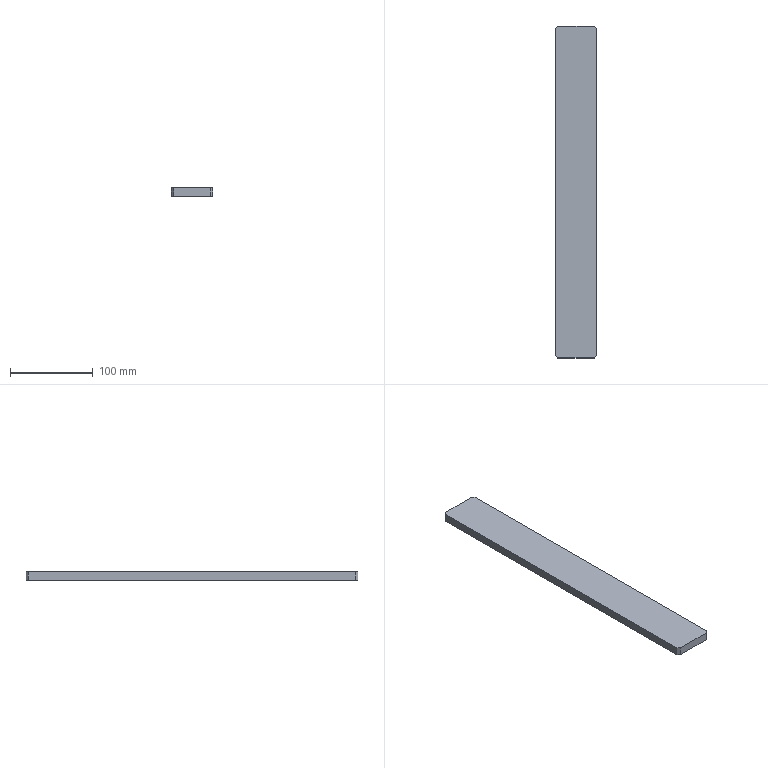Part | SolidWorks | features Chamfer 1, Extrusion 1 | 1 solid | 10 faces | box 50 x 400 x 10 mm | volume 199820 mm3 | plane 10
STEP:
#1=CARTESIAN_POINT('',(-128.557,546.194,0.));
#2=VERTEX_POINT('',#1);
#3=CARTESIAN_POINT('',(-128.557,152.194,0.));
#4=VERTEX_POINT('',#3);
#5=CARTESIAN_POINT('',(-128.557,549.194,0.));
#6=DIRECTION('',(0.,-1.,0.));
#7=VECTOR('',#6,1000.);
#8=LINE('',#5,#7);
#9=EDGE_CURVE('',#2,#4,#8,.T.);
#10=ORIENTED_EDGE('',*,*,#9,.T.);
#11=CARTESIAN_POINT('',(-128.557,152.194,10.));
#12=VERTEX_POINT('',#11);
#13=CARTESIAN_POINT('',(-128.557,152.194,10.));
#14=DIRECTION('',(0.,0.,1.));
#15=VECTOR('',#14,1000.);
#16=LINE('',#13,#15);
#17=EDGE_CURVE('',#4,#12,#16,.T.);
#18=ORIENTED_EDGE('',*,*,#17,.T.);
#19=CARTESIAN_POINT('',(-128.557,546.194,10.));
#20=VERTEX_POINT('',#19);
#21=CARTESIAN_POINT('',(-128.557,549.194,10.));
#22=DIRECTION('',(0.,-1.,0.));
#23=VECTOR('',#22,1000.);
#24=LINE('',#21,#23);
#25=EDGE_CURVE('',#20,#12,#24,.T.);
#26=ORIENTED_EDGE('',*,*,#25,.F.);
#27=CARTESIAN_POINT('',(-128.557,546.194,10.));
#28=DIRECTION('',(0.,0.,-1.));
#29=VECTOR('',#28,1000.);
#30=LINE('',#27,#29);
#31=EDGE_CURVE('',#20,#2,#30,.T.);
#32=ORIENTED_EDGE('',*,*,#31,.T.);
#33=EDGE_LOOP('',(#10,#18,#26,#32));
#34=FACE_OUTER_BOUND('',#33,.T.);
#35=CARTESIAN_POINT('',(-128.557,549.194,10.));
#36=DIRECTION('',(1.,0.,0.));
#37=DIRECTION('',(0.,1.,0.));
#38=AXIS2_PLACEMENT_3D('',#35,#36,#37);
#39=PLANE('',#38);
#40=ADVANCED_FACE('',(#34),#39,.F.);
#41=CARTESIAN_POINT('',(-125.557,149.194,0.));
#42=VERTEX_POINT('',#41);
#43=CARTESIAN_POINT('',(-81.557,149.194,0.));
#44=VERTEX_POINT('',#43);
#45=CARTESIAN_POINT('',(-128.557,149.194,0.));
#46=DIRECTION('',(1.,0.,0.));
#47=VECTOR('',#46,1000.);
#48=LINE('',#45,#47);
#49=EDGE_CURVE('',#42,#44,#48,.T.);
#50=ORIENTED_EDGE('',*,*,#49,.T.);
#51=CARTESIAN_POINT('',(-81.557,149.194,10.));
#52=VERTEX_POINT('',#51);
#53=CARTESIAN_POINT('',(-81.557,149.194,10.));
#54=DIRECTION('',(0.,0.,1.));
#55=VECTOR('',#54,1000.);
#56=LINE('',#53,#55);
#57=EDGE_CURVE('',#44,#52,#56,.T.);
#58=ORIENTED_EDGE('',*,*,#57,.T.);
#59=CARTESIAN_POINT('',(-125.557,149.194,10.));
#60=VERTEX_POINT('',#59);
#61=CARTESIAN_POINT('',(-128.557,149.194,10.));
#62=DIRECTION('',(1.,0.,0.));
#63=VECTOR('',#62,1000.);
#64=LINE('',#61,#63);
#65=EDGE_CURVE('',#60,#52,#64,.T.);
#66=ORIENTED_EDGE('',*,*,#65,.F.);
#67=CARTESIAN_POINT('',(-125.557,149.194,10.));
#68=DIRECTION('',(0.,0.,-1.));
#69=VECTOR('',#68,1000.);
#70=LINE('',#67,#69);
#71=EDGE_CURVE('',#60,#42,#70,.T.);
#72=ORIENTED_EDGE('',*,*,#71,.T.);
#73=EDGE_LOOP('',(#50,#58,#66,#72));
#74=FACE_OUTER_BOUND('',#73,.T.);
#75=CARTESIAN_POINT('',(-128.557,149.194,10.));
#76=DIRECTION('',(0.,1.,0.));
#77=DIRECTION('',(0.,0.,1.));
#78=AXIS2_PLACEMENT_3D('',#75,#76,#77);
#79=PLANE('',#78);
#80=ADVANCED_FACE('',(#74),#79,.F.);
#81=CARTESIAN_POINT('',(-78.557,152.194,10.));
#82=VERTEX_POINT('',#81);
#83=CARTESIAN_POINT('',(-78.557,546.194,10.));
#84=VERTEX_POINT('',#83);
#85=CARTESIAN_POINT('',(-78.557,549.194,10.));
#86=DIRECTION('',(0.,1.,0.));
#87=VECTOR('',#86,1000.);
#88=LINE('',#85,#87);
#89=EDGE_CURVE('',#82,#84,#88,.T.);
#90=ORIENTED_EDGE('',*,*,#89,.F.);
#91=CARTESIAN_POINT('',(-78.557,152.194,0.));
#92=VERTEX_POINT('',#91);
#93=CARTESIAN_POINT('',(-78.557,152.194,10.));
#94=DIRECTION('',(0.,0.,-1.));
#95=VECTOR('',#94,1000.);
#96=LINE('',#93,#95);
#97=EDGE_CURVE('',#82,#92,#96,.T.);
#98=ORIENTED_EDGE('',*,*,#97,.T.);
#99=CARTESIAN_POINT('',(-78.557,546.194,0.));
#100=VERTEX_POINT('',#99);
#101=CARTESIAN_POINT('',(-78.557,549.194,0.));
#102=DIRECTION('',(0.,1.,0.));
#103=VECTOR('',#102,1000.);
#104=LINE('',#101,#103);
#105=EDGE_CURVE('',#92,#100,#104,.T.);
#106=ORIENTED_EDGE('',*,*,#105,.T.);
#107=CARTESIAN_POINT('',(-78.557,546.194,10.));
#108=DIRECTION('',(0.,0.,1.));
#109=VECTOR('',#108,1000.);
#110=LINE('',#107,#109);
#111=EDGE_CURVE('',#100,#84,#110,.T.);
#112=ORIENTED_EDGE('',*,*,#111,.T.);
#113=EDGE_LOOP('',(#90,#98,#106,#112));
#114=FACE_OUTER_BOUND('',#113,.T.);
#115=CARTESIAN_POINT('',(-78.557,549.194,10.));
#116=DIRECTION('',(-1.,0.,0.));
#117=DIRECTION('',(0.,-1.,0.));
#118=AXIS2_PLACEMENT_3D('',#115,#116,#117);
#119=PLANE('',#118);
#120=ADVANCED_FACE('',(#114),#119,.F.);
#121=CARTESIAN_POINT('',(-81.557,549.194,0.));
#122=VERTEX_POINT('',#121);
#123=CARTESIAN_POINT('',(-125.557,549.194,0.));
#124=VERTEX_POINT('',#123);
#125=CARTESIAN_POINT('',(-128.557,549.194,0.));
#126=DIRECTION('',(-1.,0.,0.));
#127=VECTOR('',#126,1000.);
#128=LINE('',#125,#127);
#129=EDGE_CURVE('',#122,#124,#128,.T.);
#130=ORIENTED_EDGE('',*,*,#129,.T.);
#131=CARTESIAN_POINT('',(-125.557,549.194,10.));
#132=VERTEX_POINT('',#131);
#133=CARTESIAN_POINT('',(-125.557,549.194,10.));
#134=DIRECTION('',(0.,0.,1.));
#135=VECTOR('',#134,1000.);
#136=LINE('',#133,#135);
#137=EDGE_CURVE('',#124,#132,#136,.T.);
#138=ORIENTED_EDGE('',*,*,#137,.T.);
#139=CARTESIAN_POINT('',(-81.557,549.194,10.));
#140=VERTEX_POINT('',#139);
#141=CARTESIAN_POINT('',(-128.557,549.194,10.));
#142=DIRECTION('',(-1.,0.,0.));
#143=VECTOR('',#142,1000.);
#144=LINE('',#141,#143);
#145=EDGE_CURVE('',#140,#132,#144,.T.);
#146=ORIENTED_EDGE('',*,*,#145,.F.);
#147=CARTESIAN_POINT('',(-81.557,549.194,10.));
#148=DIRECTION('',(0.,0.,-1.));
#149=VECTOR('',#148,1000.);
#150=LINE('',#147,#149);
#151=EDGE_CURVE('',#140,#122,#150,.T.);
#152=ORIENTED_EDGE('',*,*,#151,.T.);
#153=EDGE_LOOP('',(#130,#138,#146,#152));
#154=FACE_OUTER_BOUND('',#153,.T.);
#155=CARTESIAN_POINT('',(-128.557,549.194,10.));
#156=DIRECTION('',(0.,-1.,0.));
#157=DIRECTION('',(0.,0.,-1.));
#158=AXIS2_PLACEMENT_3D('',#155,#156,#157);
#159=PLANE('',#158);
#160=ADVANCED_FACE('',(#154),#159,.F.);
#161=ORIENTED_EDGE('',*,*,#65,.T.);
#162=CARTESIAN_POINT('',(-115.375,115.375,10.));
#163=DIRECTION('',(0.7071,0.7071,0.));
#164=VECTOR('',#163,1000.);
#165=LINE('',#162,#164);
#166=EDGE_CURVE('',#52,#82,#165,.T.);
#167=ORIENTED_EDGE('',*,*,#166,.T.);
#168=ORIENTED_EDGE('',*,*,#89,.T.);
#169=CARTESIAN_POINT('',(233.818,233.818,10.));
#170=DIRECTION('',(-0.7071,0.7071,0.));
#171=VECTOR('',#170,1000.);
#172=LINE('',#169,#171);
#173=EDGE_CURVE('',#84,#140,#172,.T.);
#174=ORIENTED_EDGE('',*,*,#173,.T.);
#175=ORIENTED_EDGE('',*,*,#145,.T.);
#176=CARTESIAN_POINT('',(-337.375,337.375,10.));
#177=DIRECTION('',(-0.7071,-0.7071,0.));
#178=VECTOR('',#177,1000.);
#179=LINE('',#176,#178);
#180=EDGE_CURVE('',#132,#20,#179,.T.);
#181=ORIENTED_EDGE('',*,*,#180,.T.);
#182=ORIENTED_EDGE('',*,*,#25,.T.);
#183=CARTESIAN_POINT('',(11.818,11.818,10.));
#184=DIRECTION('',(0.7071,-0.7071,0.));
#185=VECTOR('',#184,1000.);
#186=LINE('',#183,#185);
#187=EDGE_CURVE('',#12,#60,#186,.T.);
#188=ORIENTED_EDGE('',*,*,#187,.T.);
#189=EDGE_LOOP('',(#161,#167,#168,#174,#175,#181,#182,#188));
#190=FACE_OUTER_BOUND('',#189,.T.);
#191=CARTESIAN_POINT('',(0.,0.,10.));
#192=DIRECTION('',(0.,0.,1.));
#193=DIRECTION('',(1.,0.,0.));
#194=AXIS2_PLACEMENT_3D('',#191,#192,#193);
#195=PLANE('',#194);
#196=ADVANCED_FACE('',(#190),#195,.T.);
#197=ORIENTED_EDGE('',*,*,#105,.F.);
#198=CARTESIAN_POINT('',(-78.557,152.194,0.));
#199=DIRECTION('',(-0.7071,-0.7071,0.));
#200=VECTOR('',#199,1000.);
#201=LINE('',#198,#200);
#202=EDGE_CURVE('',#92,#44,#201,.T.);
#203=ORIENTED_EDGE('',*,*,#202,.T.);
#204=ORIENTED_EDGE('',*,*,#49,.F.);
#205=CARTESIAN_POINT('',(-125.557,149.194,0.));
#206=DIRECTION('',(-0.7071,0.7071,0.));
#207=VECTOR('',#206,1000.);
#208=LINE('',#205,#207);
#209=EDGE_CURVE('',#42,#4,#208,.T.);
#210=ORIENTED_EDGE('',*,*,#209,.T.);
#211=ORIENTED_EDGE('',*,*,#9,.F.);
#212=CARTESIAN_POINT('',(-128.557,546.194,0.));
#213=DIRECTION('',(0.7071,0.7071,0.));
#214=VECTOR('',#213,1000.);
#215=LINE('',#212,#214);
#216=EDGE_CURVE('',#2,#124,#215,.T.);
#217=ORIENTED_EDGE('',*,*,#216,.T.);
#218=ORIENTED_EDGE('',*,*,#129,.F.);
#219=CARTESIAN_POINT('',(-81.557,549.194,0.));
#220=DIRECTION('',(0.7071,-0.7071,0.));
#221=VECTOR('',#220,1000.);
#222=LINE('',#219,#221);
#223=EDGE_CURVE('',#122,#100,#222,.T.);
#224=ORIENTED_EDGE('',*,*,#223,.T.);
#225=EDGE_LOOP('',(#197,#203,#204,#210,#211,#217,#218,#224));
#226=FACE_OUTER_BOUND('',#225,.T.);
#227=CARTESIAN_POINT('',(0.,0.,0.));
#228=DIRECTION('',(0.,0.,1.));
#229=DIRECTION('',(1.,0.,0.));
#230=AXIS2_PLACEMENT_3D('',#227,#228,#229);
#231=PLANE('',#230);
#232=ADVANCED_FACE('',(#226),#231,.F.);
#233=ORIENTED_EDGE('',*,*,#166,.F.);
#234=ORIENTED_EDGE('',*,*,#57,.F.);
#235=ORIENTED_EDGE('',*,*,#202,.F.);
#236=ORIENTED_EDGE('',*,*,#97,.F.);
#237=EDGE_LOOP('',(#233,#234,#235,#236));
#238=FACE_OUTER_BOUND('',#237,.T.);
#239=CARTESIAN_POINT('',(-78.557,152.194,10.));
#240=DIRECTION('',(-0.7071,0.7071,0.));
#241=DIRECTION('',(0.,0.,-1.));
#242=AXIS2_PLACEMENT_3D('',#239,#240,#241);
#243=PLANE('',#242);
#244=ADVANCED_FACE('',(#238),#243,.F.);
#245=ORIENTED_EDGE('',*,*,#187,.F.);
#246=ORIENTED_EDGE('',*,*,#17,.F.);
#247=ORIENTED_EDGE('',*,*,#209,.F.);
#248=ORIENTED_EDGE('',*,*,#71,.F.);
#249=EDGE_LOOP('',(#245,#246,#247,#248));
#250=FACE_OUTER_BOUND('',#249,.T.);
#251=CARTESIAN_POINT('',(-125.557,149.194,10.));
#252=DIRECTION('',(0.7071,0.7071,0.));
#253=DIRECTION('',(0.,0.,-1.));
#254=AXIS2_PLACEMENT_3D('',#251,#252,#253);
#255=PLANE('',#254);
#256=ADVANCED_FACE('',(#250),#255,.F.);
#257=ORIENTED_EDGE('',*,*,#180,.F.);
#258=ORIENTED_EDGE('',*,*,#137,.F.);
#259=ORIENTED_EDGE('',*,*,#216,.F.);
#260=ORIENTED_EDGE('',*,*,#31,.F.);
#261=EDGE_LOOP('',(#257,#258,#259,#260));
#262=FACE_OUTER_BOUND('',#261,.T.);
#263=CARTESIAN_POINT('',(-128.557,546.194,10.));
#264=DIRECTION('',(0.7071,-0.7071,0.));
#265=DIRECTION('',(0.,0.,-1.));
#266=AXIS2_PLACEMENT_3D('',#263,#264,#265);
#267=PLANE('',#266);
#268=ADVANCED_FACE('',(#262),#267,.F.);
#269=ORIENTED_EDGE('',*,*,#173,.F.);
#270=ORIENTED_EDGE('',*,*,#111,.F.);
#271=ORIENTED_EDGE('',*,*,#223,.F.);
#272=ORIENTED_EDGE('',*,*,#151,.F.);
#273=EDGE_LOOP('',(#269,#270,#271,#272));
#274=FACE_OUTER_BOUND('',#273,.T.);
#275=CARTESIAN_POINT('',(-81.557,549.194,10.));
#276=DIRECTION('',(-0.7071,-0.7071,0.));
#277=DIRECTION('',(0.,0.,-1.));
#278=AXIS2_PLACEMENT_3D('',#275,#276,#277);
#279=PLANE('',#278);
#280=ADVANCED_FACE('',(#274),#279,.F.);
#281=CLOSED_SHELL('',(#40,#80,#120,#160,#196,#232,#244,#256,#268,#280));
#282=MANIFOLD_SOLID_BREP('',#281);
#283=CARTESIAN_POINT('',(0.,0.,0.));
#284=DIRECTION('',(0.,0.,1.));
#285=DIRECTION('',(1.,0.,0.));
#286=AXIS2_PLACEMENT_3D('',#283,#284,#285);
#287=(LENGTH_UNIT()NAMED_UNIT(*)SI_UNIT(.MILLI.,.METRE.));
#288=UNCERTAINTY_MEASURE_WITH_UNIT(LENGTH_MEASURE(0.00001),#287,'','');
#289=(NAMED_UNIT(*)PLANE_ANGLE_UNIT()SI_UNIT($,.RADIAN.));
#290=(NAMED_UNIT(*)SI_UNIT($,.STERADIAN.)SOLID_ANGLE_UNIT());
#291=(GEOMETRIC_REPRESENTATION_CONTEXT(3)GLOBAL_UNCERTAINTY_ASSIGNED_CONTEXT((#288))GLOBAL_UNIT_ASSIGNED_CONTEXT((#287,#289,#290))REPRESENTATION_CONTEXT('',''));
#292=ADVANCED_BREP_SHAPE_REPRESENTATION('',(#282,#286),#291);